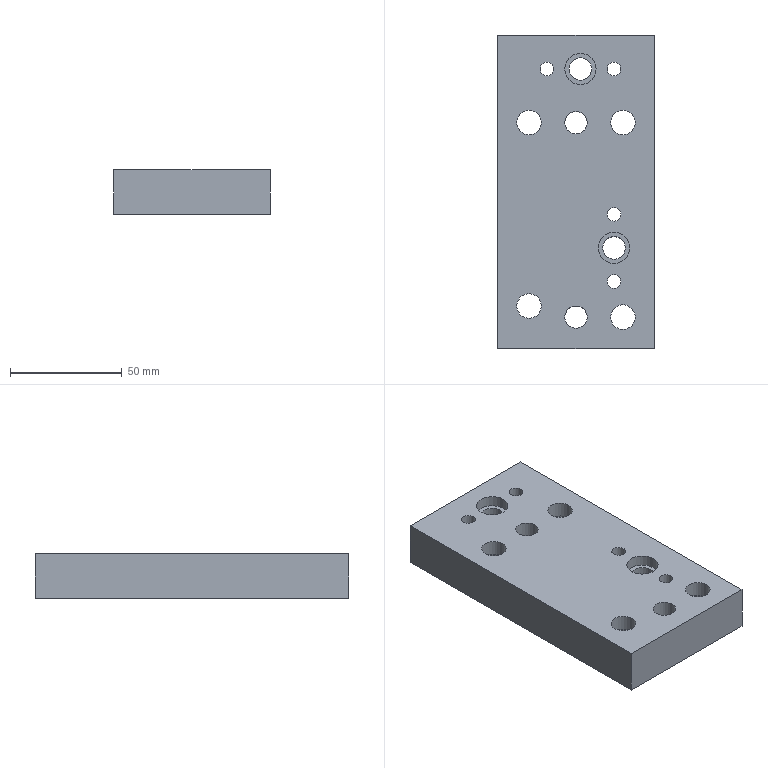Part | STEP file | 407_id2722_x_t | 1 solid | 34 faces | box 70 x 140 x 20 mm | volume 171561 mm3 | cylinder 20 | plane 14 | commonest cylinder face diameters 6.1 x4 11 x4 17 x4 10 x2 10.1 x2 12 x2